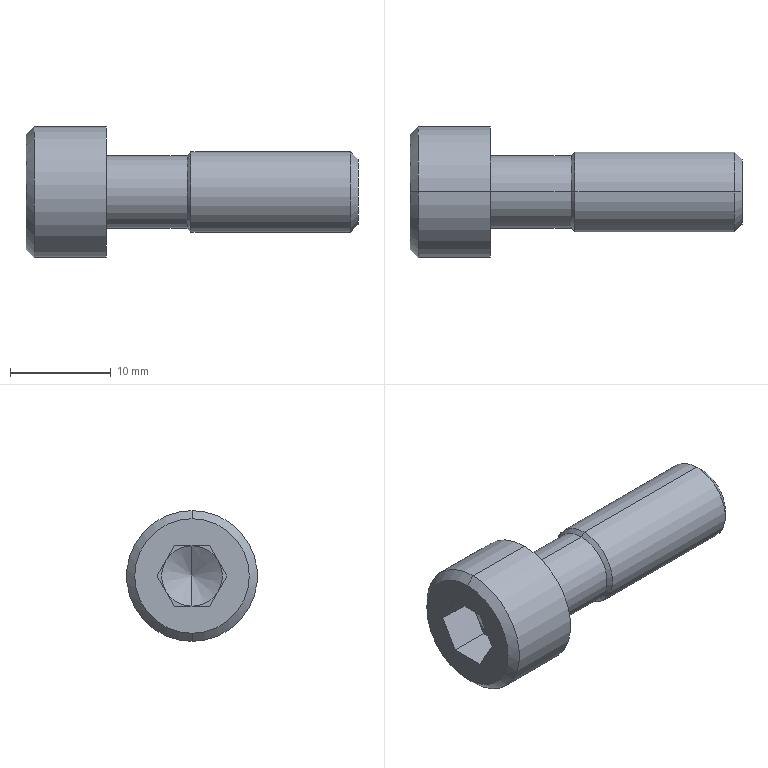Part | STEP file | 0243_Z_SCBS8-25_1 | 1 solid | 29 faces | box 33 x 13 x 13 mm | volume 2083 mm3 | plane 15 | cone 8 | cylinder 6 | commonest cylinder face diameters 7.232 x2 8 x2 13 x2